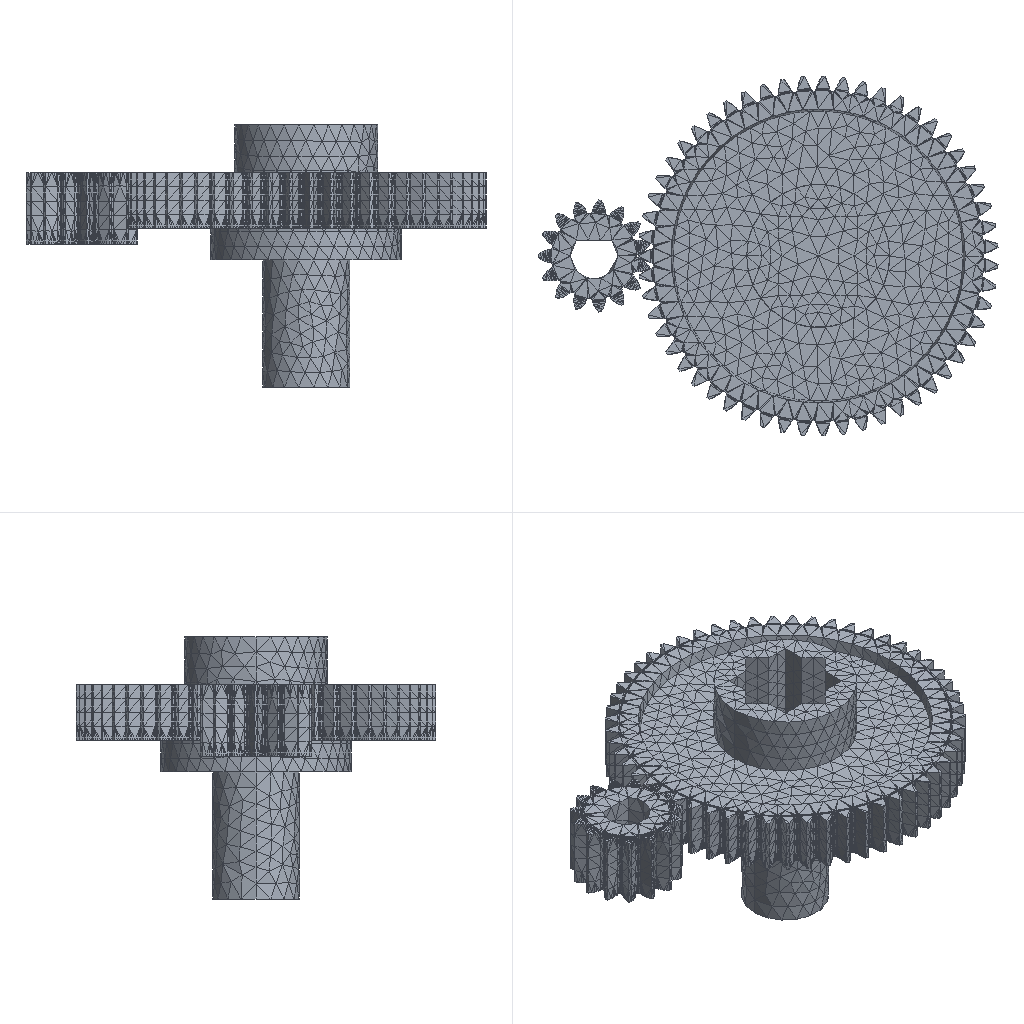Simulation study | ansys workbench
Set-up summary:
category,name,step,type,value,unit,region
solver,ansys_mapdl
solver,version,,,22.1
solver,version,,,22.1
units,MPA,,stated
analysis,deck1,,static,static
load_step,requested,,,1
analysis,nlgeom
mesh,nodes,,,42283
mesh,elements,,,24210
element_type,ANSYS 187 (type 1)
element_type,ANSYS 187 (type 2)
element_type,ANSYS 174 (type 3)
element_type,ANSYS 170 (type 4)
element_type,ANSYS 174 (type 5)
element_type,ANSYS 170 (type 6)
element_type,ANSYS 174 (type 7)
element_type,ANSYS 170 (type 8)
load,load commands in deck,,count,6
bc,support commands in deck,,count,1
named_set,A,,component
named_set,C_2,,component
named_set,_FIXEDSU,,component
named_set,______,,component
analysis,deck2,,static,static
load_step,requested,,,1
analysis,nlgeom
mesh,nodes,,,42283
mesh,elements,,,24210
element_type,ANSYS 187 (type 1)
element_type,ANSYS 187 (type 2)
element_type,ANSYS 174 (type 3)
element_type,ANSYS 170 (type 4)
element_type,ANSYS 174 (type 5)
element_type,ANSYS 170 (type 6)
element_type,ANSYS 174 (type 7)
element_type,ANSYS 170 (type 8)
load,load commands in deck,,count,6
bc,support commands in deck,,count,1
named_set,A,,component
named_set,C_2,,component
named_set,_FIXEDSU,,component
named_set,______,,component
material,1,,in results
material,2,,in results
material,1,,in results
material,2,,in results
check,setup vs results,,match,results also hold 2 node(s) and 2 element(s) the deck makes with ['EN']; those were not compared
check,setup vs results,,match,results also hold 2 node(s) and 2 element(s) the deck makes with ['EN']; those were not compared
Ansys APDL input file, long lists of numbers shortened:
/batch
/config,noeldb,1     ! force off writing results to database
*get,_wallstrt,active,,time,wall
! ANSYS input file written by Workbench version 2022 R1
! File used for geometry attach: F:\____________________\____________________\_______.STEP
/title,wbnew--____ (B5)
! ****** Begin Custom Load Command Snippet ******
/COM, ACT Extensions:
/COM,     LSDYNA, 2021.1
/COM,
! ****** End   Custom Load Command Snippet ******
*DIM,_wb_ProjectScratch_dir,string,248
_wb_ProjectScratch_dir(1) = 'C:\_____\_____________\_______\_____\____\_______________________\_______________\_______\_
*DIM,_wb_SolverFiles_dir,string,248
_wb_SolverFiles_dir(1) = 'C:\_____\_____________\_______\_____\____\_______________________\___________\___\___\____\_
*DIM,_wb_userfiles_dir,string,248
_wb_userfiles_dir(1) = 'C:\_____\_____________\_______\_____\____\_______________________\___________\__________\_
/com,--- Data in consistent NMM units. See Solving Units in the help system for more information.
/units,MPA
/nopr
/wb,file,start              !  signify a WB generated input file
/prep7
! Turn off shape checking because checks already performed inside WB mesher.
! See help system for more information.
SHPP,OFF,,NOWARN
/nolist
etcon,set             ! allow ANSYS to choose best KEYOP's for 180x elements, resets any applicable keyopt to MAPDL defaults
/com,*********** Nodes for the whole assembly ***********
nblock,3,,46509
(1i9,3e20.9e3)
        1    -5.324198798E+01    -1.723703329E+02     9.955000000E+02
! (42280 more lines like these left out)
-1
/com,*********** Nodes for all Remote Points ***********
nblock,3
(1i9,3e20.9e3)
    42282    -5.086632081E+01    -1.744100114E+02     9.977502952E+02
    42283    -3.790070204E+01    -1.748059206E+02     9.982495383E+02
-1
/wb,elem,start            !  set before creation of elements
/com,*********** Elements for Body 1 "15T|Admi1DC8396Chgo2[1]" ***********
et,1,187
eblock,19,solid,,4124
(19i9)
        1        1        1        1        0        0        0        0       10        0        1      890     1352     1243     1283     6212     7776     6208     6211
! (8247 more lines like these left out)
-1
/com,*********** Elements for Body 2 "55T__|NONE" ***********
et,2,187
eblock,19,solid,,18188
(19i9)
        2        2        2        2        0        0        0        0       10        0     4125    12426    12434    13675    13632    38243    38308    38251    38250
! (36375 more lines like these left out)
-1
/wb,elem,end               !  done creating elements
/com,*********** Send User Defined Coordinate System(s) ***********
csys,0
toffst,273.15,  ! Temperature offset from absolute zero
/com,*********** Set Reference Temperature ***********
tref,22.
/wb,mat,start              !  starting to send materials
/com,*********** Send Materials ***********
Temperature = 'TEMP' ! Temperature
MP,DENS,1,7.85e-09,	! tonne mm^-3
MP,ALPX,1,1.2e-05,	! C^-1
MP,C,1,434000000,	! mm^2 s^-2 C^-1
MP,KXX,1,60.5,	! tonne mm s^-3 C^-1
MP,RSVX,1,0.00017,	! ohm mm
MP,EX,1,200000,	! tonne s^-2 mm^-1
MP,NUXY,1,0.3,
MP,MURX,1,10000,
Temperature = 'TEMP' ! Temperature
MP,DENS,2,7.85e-09,	! tonne mm^-3
MP,ALPX,2,1.2e-05,	! C^-1
MP,C,2,434000000,	! mm^2 s^-2 C^-1
MP,KXX,2,60.5,	! tonne mm s^-3 C^-1
MP,RSVX,2,0.00017,	! ohm mm
MP,EX,2,200000,	! tonne s^-2 mm^-1
MP,NUXY,2,0.3,
MP,MURX,2,10000,
/wb,mat,end                !  done sending materials
!************************* Model Summary ********************
!15T|Admi1DC8396Chgo2[1], Structural Steel, matid, 1
!55T__|NONE, Structural Steel, matid, 2
!************************* End Model Summary ********************
! get the diagonal of the bounding box. Needed later for other things
*get,_xmin,node,,mnloc,x
*get,_ymin,node,,mnloc,y
*get,_zmin,node,,mnloc,z
*get,_xmax,node,,mxloc,x
*get,_ymax,node,,mxloc,y
*get,_zmax,node,,mxloc,z
_ASMDIAG=(_xmax-_xmin)*(_xmax-_xmin)+(_ymax-_ymin)*(_ymax-_ymin)+(_zmax-_zmin)*(_zmax-_zmin)
_ASMDIAG=SQRT(_ASMDIAG)
/wb,contact,start          !  starting to send contact
/com,*********** Create Contact "Contact Region" ***********
/com,            Real Constant Set For Above Contact Is 4 & 3
*set,tid,4
*set,cid,3
r,tid
r,cid
et,tid,170
et,cid,174
eblock,10,,,84
(15i9)
    34027        4        4        4        0      237      241      242      242     3025     3046      242     3026
! (83 more lines like these left out)
-1
eblock,10,,,84
(15i9)
    34111        3        3        3        0      237      241      242      242     3025     3046      242     3026
! (83 more lines like these left out)
-1
eblock,10,,,52
(15i9)
    34195        3        4        3        0    11025    11014    11026    11026    29709    29710    11026    29766
! (51 more lines like these left out)
-1
eblock,10,,,52
(15i9)
    34247        4        3        4        0    11025    11014    11026    11026    29709    29710    11026    29766
! (51 more lines like these left out)
-1
keyo,cid,8,2               ! auto create asymmetric contact (from Program Controlled setting)
keyo,cid,10,0              ! adjust contact stiffness each NR iteration (from Program Controlled setting)
keyo,cid,12,5              ! bonded always
keyo,cid,18,1              ! small sliding turned on by application
keyo,cid,2,0               ! augmented Lagrange (from Program Controlled setting)
keyo,cid,4,0               ! on Gauss point (from Program Controlled setting)
keyo,cid,9,1               ! ignore initial gaps/penetration
keyo,cid,7,0               ! No Prediction
rmod,tid,3,10.      ! FKN
rmod,tid,5,0.       ! ICONT
rmod,tid,6,0.       ! PINB
rmod,tid,10,0.      ! CNOF
rmod,tid,12,0.      ! FKT
rmod,tid,36,29      ! WB DSID
rmod,cid,3,10.      ! FKN
rmod,cid,5,0.       ! ICONT
rmod,cid,6,0.       ! PINB
rmod,cid,10,0.      ! CNOF
rmod,cid,12,0.      ! FKT
rmod,cid,36,29      ! WB DSID
nsel,all
esel,all
/wb,contact,end            !  done creating contacts
/com,*********** Send Named Selection as Node Component ***********
CMBLOCK,______  ,NODE,     1116
(8i10)
        86        87        88        89        90        91        92        93
! (139 more lines like these left out)
/com,*********** Send Named Selection as Node Component ***********
CMBLOCK,A       ,NODE,      599
(8i10)
       180       181       182       183       184       185       186       187
! (74 more lines like these left out)
/com,*********** Send Named Selection as Node Component ***********
CMBLOCK,C_2     ,NODE,     4620
(8i10)
      7978      7980      7981      7982      7983      7984      7985      7992
! (577 more lines like these left out)
/golist
/wb,load,start             !  starting to send loads
/com,*********** Fixed Supports ***********
CMBLOCK,_FIXEDSU,NODE,     1116
(8i10)
        86        87        88        89        90        91        92        93
! (139 more lines like these left out)
cmsel,s,_FIXEDSU
d,all,all
nsel,all
/com,*********** Create Remote Point "Internal Remote Point" ***********
! -------- Remote Point Used by "Moment" --------
*set,tid,6
*set,cid,5
et,cid,174
et,tid,170
keyo,tid,2,1               ! Don't fix the pilot node
keyo,tid,4,111111
keyo,cid,12,5              ! Bonded Contact
keyo,cid,4,1               ! Deformable RBE3 style load
keyo,cid,2,2               ! MPC style contact
eblock,10,,,196
(15i9)
    34299        5        5        5        0      184      196      195      195     2758     2820      195     2757
! (195 more lines like these left out)
-1
*set,_npilot,42282
_npilot45=_npilot
type,tid
mat ,cid
real,cid
tshape,pilo
en,34495,_npilot
tshape
/com,*********** Create Remote Point "Internal Remote Point 2" ***********
! -------- Remote Point Used by "Moment 2" --------
*set,tid,8
*set,cid,7
et,cid,174
et,tid,170
keyo,tid,2,1               ! Don't fix the pilot node
keyo,tid,4,111111
keyo,cid,12,5              ! Bonded Contact
keyo,cid,4,1               ! Deformable RBE3 style load
keyo,cid,2,2               ! MPC style contact
eblock,10,,,1430
(15i9)
    34496        7        7        7        0     9141    11045     9142     9142    19272    19274     9142    19270
! (1429 more lines like these left out)
-1
*set,_npilot,42283
_npilot59=_npilot
type,tid
mat ,cid
real,cid
tshape,pilo
en,35926,_npilot
tshape
/com,*********** Construct Moment Using Remote Attachment ***********
/com,*********** Construct Moment Using Remote Attachment ***********
/gst,on,on
fini
*get,_numnode,node,0,count
*get,_numelem,elem,0,count
*get, _MAXELEMNUM, elem, 0, NUM, MAX
*get, _MAXNODENUM, node, 0, NUM, MAX
*get, _MAXELEMTYPE, etyp, 0, NUM, MAX
*get, _MAXREALCONST, real, 0, NUM, MAX
/go
/wb,load,end               !  done creating loads
/com,--- Number of total nodes = %_numnode%
/com,--- Number of contact elements = 1898
/com,--- Number of spring elements = 0
/com,--- Number of bearing elements = 0
/com,--- Number of solid elements = 22312
/com,--- Number of condensed parts = 0
/com,--- Number of total elements = %_numelem%
*get,_wallbsol,active,,time,wall
/com,****************************************************************************
/com,*************************    SOLUTION       ********************************
/com,****************************************************************************
/solu
antype,0                   ! static analysis
_thickRatio=  1     ! Ratio of thick parts in the model
eqsl,pcg,1e-8,,,,,,1
cntr,print,1               ! print out contact info and also make no initial contact an error
dmpoption,emat,no             ! Don't combine emat file for DANSYS
dmpoption,esav,no             ! Don't combine esav file for DANSYS
nldiag,cont,iter           ! print out contact info each equilibrium iteration
rescontrol,,none                 ! Do not keep any restart files
/com,****************************************************
/com,******************* SOLVE FOR LS 1 OF 1 ****************
nsel,s,node,,42282
f,all,mx,0.
f,all,my,0.
f,all,mz,127.6
nsel,s,node,,42283
f,all,mx,0.
f,all,my,0.
f,all,mz,-468.
nsel,all
/nopr
/gopr
nsub,1,1,1
time,1.
outres,erase
outres,all,none
outres,nsol,all,
outres,rsol,all
outres,eangl,all
outres,etmp,all
outres,veng,all
outres,strs,all,
outres,epel,all,
outres,eppl,all,
outres,cont,all,
! *********** WB SOLVE COMMAND ***********
! check interactive state
*get,ANSINTER_,active,,int
*if,ANSINTER_,ne,0,then
/eof
*endif
solve
/com *************** Write FE CONNECTORS *********
CEWRITE,file,ce,,INTE
/com,****************************************************
/com,*************** FINISHED SOLVE FOR LS 1 *************
*get,_wallasol,active,,time,wall
/nopr
*get,_numnode,node,0,count
*get,_numelem,elem,0,count
*get, _MAXELEMNUM, elem, 0, NUM, MAX
*get, _MAXNODENUM, node, 0, NUM, MAX,,,INTERNAL
*get, _MAXELEMTYPE, etyp, 0, NUM, MAX
*get, _MAXREALCONST, real, 0, NUM, MAX
/gopr
*get,_PCGITER,active,,solu,cgiter
/post1
xmlo,ENCODING,ISO-8859-1
xmlo,parm
/xml,parm,xml
fini
/gopr
*get,_walldone,active,,time,wall
_preptime=(_wallbsol-_wallstrt)*3600
_solvtime=(_wallasol-_wallbsol)*3600
_posttime=(_walldone-_wallasol)*3600
_totaltim=(_walldone-_wallstrt)*3600
*get,_dlbratio,active,0,solu,dlbr
*get,_combtime,active,0,solu,comb
*get,_ssmode,active,0,solu,ssmm
*get,_ndofs,active,0,solu,ndof
*get,_sol_end_time,active,0,set,time
*if,_sol_end_time,eq,1.,then
/fclean				!clean distributed files
*endif
/com,--- Total number of nodes = %_numnode%
/com,--- Total number of elements = %_numelem%
/com,--- Element load balance ratio = %_dlbratio%
/com,--- Time to combine distributed files = %_combtime%
/com,--- Sparse memory mode = %_ssmode%
/com,--- Number of DOF = %_ndofs%
/wb,file,end               ! done with WB generated input
Results summary:
result,analysis,,,static
result,last_loadstep,,,1
result,primary field,,,displacement
result,reaction total,1,FX,0.0,N
result,reaction total,1,FY,0.0,N
result,reaction total,1,FZ,0.0,N
result,mass,,,1.2e-05,"NMM: mm, ton, N, s, mV, mA, degC"
result,analysis,,,static
result,last_loadstep,,,1
result,primary field,,,displacement
result,reaction total,1,FX,0.0,N
result,reaction total,1,FY,0.0,N
result,reaction total,1,FZ,0.0,N
result,mass,,,2e-06,"NMM: mm, ton, N, s, mV, mA, degC"